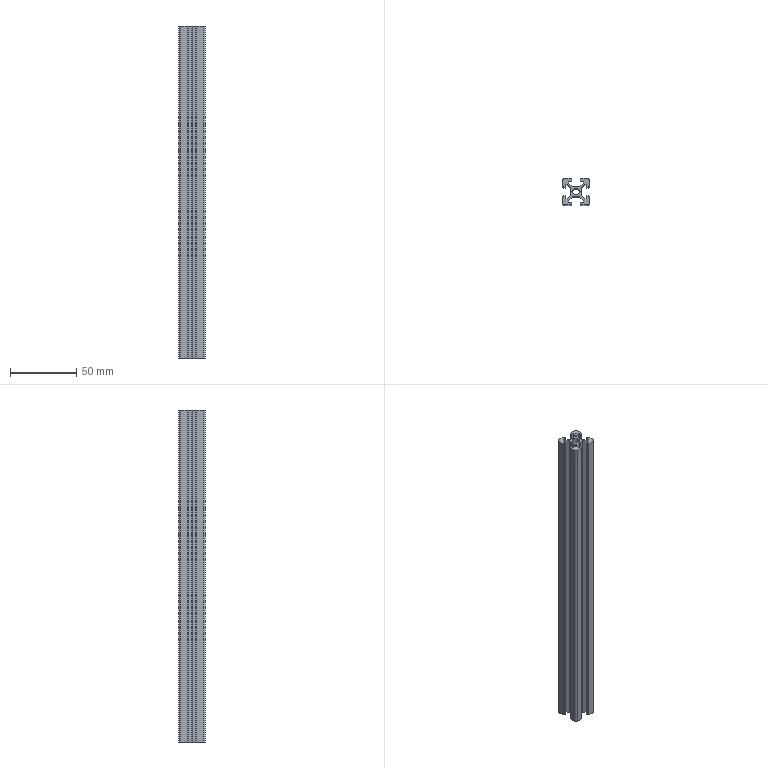Part | STEP file | AOB02-H2020_YHD018 | 1 solid | 80 faces | box 20 x 20 x 251 mm | volume 43333 mm3 | plane 74 | cylinder 6 | commonest cylinder face diameters 3 x4 5 x2